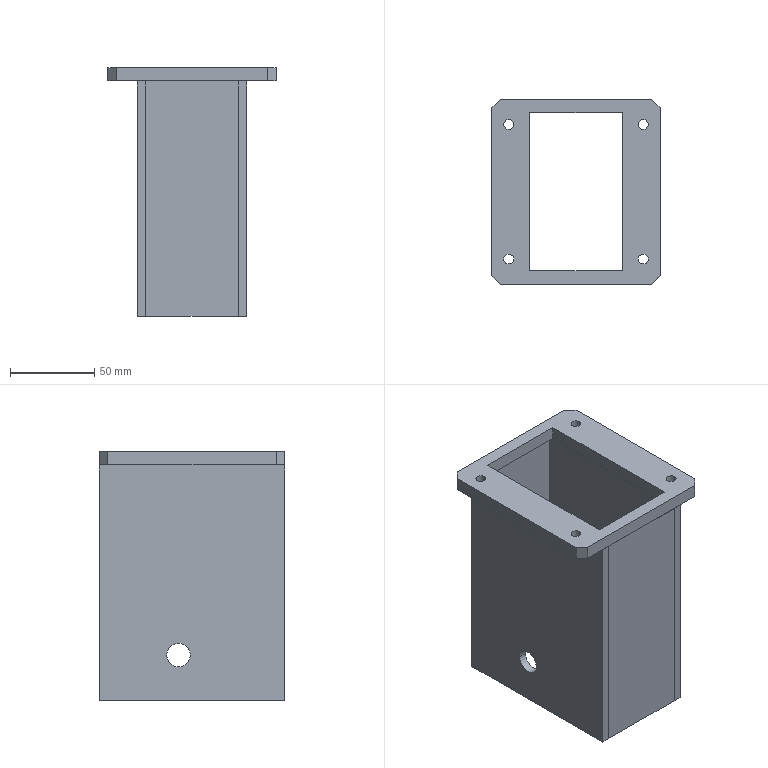Part | SolidWorks | features ICE 4, Chamfer 1, Extrusion 1, HoleWzd 1 | 5 solids | 50 faces | box 100 x 110 x 148 mm | volume 274855 mm3 | plane 38 | cylinder 12 | commonest cylinder face diameters 5.8 x8 14 x4
STEP:
#1=CARTESIAN_POINT('',(27.5,55.,0.));
#2=VERTEX_POINT('',#1);
#3=CARTESIAN_POINT('',(27.5,50.,0.));
#4=VERTEX_POINT('',#3);
#5=CARTESIAN_POINT('',(27.5,50.,0.));
#6=DIRECTION('',(0.,-1.,0.));
#7=VECTOR('',#6,1000.);
#8=LINE('',#5,#7);
#9=EDGE_CURVE('',#2,#4,#8,.T.);
#10=ORIENTED_EDGE('',*,*,#9,.T.);
#11=CARTESIAN_POINT('',(27.5,50.,-140.));
#12=VERTEX_POINT('',#11);
#13=CARTESIAN_POINT('',(27.5,50.,-140.));
#14=DIRECTION('',(0.,0.,1.));
#15=VECTOR('',#14,1000.);
#16=LINE('',#13,#15);
#17=EDGE_CURVE('',#12,#4,#16,.T.);
#18=ORIENTED_EDGE('',*,*,#17,.F.);
#19=CARTESIAN_POINT('',(27.5,55.,-140.));
#20=VERTEX_POINT('',#19);
#21=CARTESIAN_POINT('',(27.5,50.,-140.));
#22=DIRECTION('',(0.,-1.,0.));
#23=VECTOR('',#22,1000.);
#24=LINE('',#21,#23);
#25=EDGE_CURVE('',#20,#12,#24,.T.);
#26=ORIENTED_EDGE('',*,*,#25,.F.);
#27=CARTESIAN_POINT('',(27.5,55.,-140.));
#28=DIRECTION('',(0.,0.,1.));
#29=VECTOR('',#28,1000.);
#30=LINE('',#27,#29);
#31=EDGE_CURVE('',#20,#2,#30,.T.);
#32=ORIENTED_EDGE('',*,*,#31,.T.);
#33=EDGE_LOOP('',(#10,#18,#26,#32));
#34=FACE_OUTER_BOUND('',#33,.T.);
#35=CARTESIAN_POINT('',(27.5,50.,-140.));
#36=DIRECTION('',(-1.,0.,0.));
#37=DIRECTION('',(0.,-1.,0.));
#38=AXIS2_PLACEMENT_3D('',#35,#36,#37);
#39=PLANE('',#38);
#40=ADVANCED_FACE('',(#34),#39,.F.);
#41=CARTESIAN_POINT('',(-27.5,50.,0.));
#42=VERTEX_POINT('',#41);
#43=CARTESIAN_POINT('',(27.5,50.,0.));
#44=DIRECTION('',(-1.,0.,0.));
#45=VECTOR('',#44,1000.);
#46=LINE('',#43,#45);
#47=EDGE_CURVE('',#4,#42,#46,.T.);
#48=ORIENTED_EDGE('',*,*,#47,.T.);
#49=CARTESIAN_POINT('',(-27.5,50.,-140.));
#50=VERTEX_POINT('',#49);
#51=CARTESIAN_POINT('',(-27.5,50.,-140.));
#52=DIRECTION('',(0.,0.,1.));
#53=VECTOR('',#52,1000.);
#54=LINE('',#51,#53);
#55=EDGE_CURVE('',#50,#42,#54,.T.);
#56=ORIENTED_EDGE('',*,*,#55,.F.);
#57=CARTESIAN_POINT('',(27.5,50.,-140.));
#58=DIRECTION('',(-1.,0.,0.));
#59=VECTOR('',#58,1000.);
#60=LINE('',#57,#59);
#61=EDGE_CURVE('',#12,#50,#60,.T.);
#62=ORIENTED_EDGE('',*,*,#61,.F.);
#63=ORIENTED_EDGE('',*,*,#17,.T.);
#64=EDGE_LOOP('',(#48,#56,#62,#63));
#65=FACE_OUTER_BOUND('',#64,.T.);
#66=CARTESIAN_POINT('',(27.5,50.,-140.));
#67=DIRECTION('',(0.,1.,0.));
#68=DIRECTION('',(0.,0.,1.));
#69=AXIS2_PLACEMENT_3D('',#66,#67,#68);
#70=PLANE('',#69);
#71=ADVANCED_FACE('',(#65),#70,.F.);
#72=CARTESIAN_POINT('',(-27.5,55.,0.));
#73=VERTEX_POINT('',#72);
#74=CARTESIAN_POINT('',(-27.5,50.,0.));
#75=DIRECTION('',(0.,1.,0.));
#76=VECTOR('',#75,1000.);
#77=LINE('',#74,#76);
#78=EDGE_CURVE('',#42,#73,#77,.T.);
#79=ORIENTED_EDGE('',*,*,#78,.T.);
#80=CARTESIAN_POINT('',(-27.5,55.,-140.));
#81=VERTEX_POINT('',#80);
#82=CARTESIAN_POINT('',(-27.5,55.,-140.));
#83=DIRECTION('',(0.,0.,1.));
#84=VECTOR('',#83,1000.);
#85=LINE('',#82,#84);
#86=EDGE_CURVE('',#81,#73,#85,.T.);
#87=ORIENTED_EDGE('',*,*,#86,.F.);
#88=CARTESIAN_POINT('',(-27.5,50.,-140.));
#89=DIRECTION('',(0.,1.,0.));
#90=VECTOR('',#89,1000.);
#91=LINE('',#88,#90);
#92=EDGE_CURVE('',#50,#81,#91,.T.);
#93=ORIENTED_EDGE('',*,*,#92,.F.);
#94=ORIENTED_EDGE('',*,*,#55,.T.);
#95=EDGE_LOOP('',(#79,#87,#93,#94));
#96=FACE_OUTER_BOUND('',#95,.T.);
#97=CARTESIAN_POINT('',(-27.5,50.,-140.));
#98=DIRECTION('',(1.,0.,0.));
#99=DIRECTION('',(0.,0.,-1.));
#100=AXIS2_PLACEMENT_3D('',#97,#98,#99);
#101=PLANE('',#100);
#102=ADVANCED_FACE('',(#96),#101,.F.);
#103=CARTESIAN_POINT('',(27.5,55.,0.));
#104=DIRECTION('',(1.,0.,0.));
#105=VECTOR('',#104,1000.);
#106=LINE('',#103,#105);
#107=EDGE_CURVE('',#73,#2,#106,.T.);
#108=ORIENTED_EDGE('',*,*,#107,.T.);
#109=ORIENTED_EDGE('',*,*,#31,.F.);
#110=CARTESIAN_POINT('',(27.5,55.,-140.));
#111=DIRECTION('',(1.,0.,0.));
#112=VECTOR('',#111,1000.);
#113=LINE('',#110,#112);
#114=EDGE_CURVE('',#81,#20,#113,.T.);
#115=ORIENTED_EDGE('',*,*,#114,.F.);
#116=ORIENTED_EDGE('',*,*,#86,.T.);
#117=EDGE_LOOP('',(#108,#109,#115,#116));
#118=FACE_OUTER_BOUND('',#117,.T.);
#119=CARTESIAN_POINT('',(27.5,55.,-140.));
#120=DIRECTION('',(0.,-1.,0.));
#121=DIRECTION('',(0.,0.,-1.));
#122=AXIS2_PLACEMENT_3D('',#119,#120,#121);
#123=PLANE('',#122);
#124=ADVANCED_FACE('',(#118),#123,.F.);
#125=ORIENTED_EDGE('',*,*,#25,.T.);
#126=ORIENTED_EDGE('',*,*,#61,.T.);
#127=ORIENTED_EDGE('',*,*,#92,.T.);
#128=ORIENTED_EDGE('',*,*,#114,.T.);
#129=EDGE_LOOP('',(#125,#126,#127,#128));
#130=FACE_OUTER_BOUND('',#129,.T.);
#131=CARTESIAN_POINT('',(0.,0.,-140.));
#132=DIRECTION('',(0.,0.,1.));
#133=DIRECTION('',(1.,0.,0.));
#134=AXIS2_PLACEMENT_3D('',#131,#132,#133);
#135=PLANE('',#134);
#136=ADVANCED_FACE('',(#130),#135,.F.);
#137=ORIENTED_EDGE('',*,*,#9,.F.);
#138=ORIENTED_EDGE('',*,*,#107,.F.);
#139=ORIENTED_EDGE('',*,*,#78,.F.);
#140=ORIENTED_EDGE('',*,*,#47,.F.);
#141=EDGE_LOOP('',(#137,#138,#139,#140));
#142=FACE_OUTER_BOUND('',#141,.T.);
#143=CARTESIAN_POINT('',(0.,0.,0.));
#144=DIRECTION('',(0.,0.,1.));
#145=DIRECTION('',(1.,0.,0.));
#146=AXIS2_PLACEMENT_3D('',#143,#144,#145);
#147=PLANE('',#146);
#148=ADVANCED_FACE('',(#142),#147,.T.);
#149=CLOSED_SHELL('',(#40,#71,#102,#124,#136,#148));
#150=MANIFOLD_SOLID_BREP('',#149);
#151=CARTESIAN_POINT('',(-27.5,-50.,0.));
#152=VERTEX_POINT('',#151);
#153=CARTESIAN_POINT('',(27.5,-50.,0.));
#154=VERTEX_POINT('',#153);
#155=CARTESIAN_POINT('',(27.5,-50.,0.));
#156=DIRECTION('',(1.,0.,0.));
#157=VECTOR('',#156,1000.);
#158=LINE('',#155,#157);
#159=EDGE_CURVE('',#152,#154,#158,.T.);
#160=ORIENTED_EDGE('',*,*,#159,.T.);
#161=CARTESIAN_POINT('',(27.5,-50.,-140.));
#162=VERTEX_POINT('',#161);
#163=CARTESIAN_POINT('',(27.5,-50.,-140.));
#164=DIRECTION('',(0.,0.,1.));
#165=VECTOR('',#164,1000.);
#166=LINE('',#163,#165);
#167=EDGE_CURVE('',#162,#154,#166,.T.);
#168=ORIENTED_EDGE('',*,*,#167,.F.);
#169=CARTESIAN_POINT('',(-27.5,-50.,-140.));
#170=VERTEX_POINT('',#169);
#171=CARTESIAN_POINT('',(27.5,-50.,-140.));
#172=DIRECTION('',(1.,0.,0.));
#173=VECTOR('',#172,1000.);
#174=LINE('',#171,#173);
#175=EDGE_CURVE('',#170,#162,#174,.T.);
#176=ORIENTED_EDGE('',*,*,#175,.F.);
#177=CARTESIAN_POINT('',(-27.5,-50.,-140.));
#178=DIRECTION('',(0.,0.,1.));
#179=VECTOR('',#178,1000.);
#180=LINE('',#177,#179);
#181=EDGE_CURVE('',#170,#152,#180,.T.);
#182=ORIENTED_EDGE('',*,*,#181,.T.);
#183=EDGE_LOOP('',(#160,#168,#176,#182));
#184=FACE_OUTER_BOUND('',#183,.T.);
#185=CARTESIAN_POINT('',(27.5,-50.,-140.));
#186=DIRECTION('',(0.,-1.,0.));
#187=DIRECTION('',(0.,0.,-1.));
#188=AXIS2_PLACEMENT_3D('',#185,#186,#187);
#189=PLANE('',#188);
#190=ADVANCED_FACE('',(#184),#189,.F.);
#191=CARTESIAN_POINT('',(27.5,-55.,0.));
#192=VERTEX_POINT('',#191);
#193=CARTESIAN_POINT('',(27.5,-50.,0.));
#194=DIRECTION('',(0.,-1.,0.));
#195=VECTOR('',#194,1000.);
#196=LINE('',#193,#195);
#197=EDGE_CURVE('',#154,#192,#196,.T.);
#198=ORIENTED_EDGE('',*,*,#197,.T.);
#199=CARTESIAN_POINT('',(27.5,-55.,-140.));
#200=VERTEX_POINT('',#199);
#201=CARTESIAN_POINT('',(27.5,-55.,-140.));
#202=DIRECTION('',(0.,0.,1.));
#203=VECTOR('',#202,1000.);
#204=LINE('',#201,#203);
#205=EDGE_CURVE('',#200,#192,#204,.T.);
#206=ORIENTED_EDGE('',*,*,#205,.F.);
#207=CARTESIAN_POINT('',(27.5,-50.,-140.));
#208=DIRECTION('',(0.,-1.,0.));
#209=VECTOR('',#208,1000.);
#210=LINE('',#207,#209);
#211=EDGE_CURVE('',#162,#200,#210,.T.);
#212=ORIENTED_EDGE('',*,*,#211,.F.);
#213=ORIENTED_EDGE('',*,*,#167,.T.);
#214=EDGE_LOOP('',(#198,#206,#212,#213));
#215=FACE_OUTER_BOUND('',#214,.T.);
#216=CARTESIAN_POINT('',(27.5,-50.,-140.));
#217=DIRECTION('',(-1.,0.,0.));
#218=DIRECTION('',(0.,0.,1.));
#219=AXIS2_PLACEMENT_3D('',#216,#217,#218);
#220=PLANE('',#219);
#221=ADVANCED_FACE('',(#215),#220,.F.);
#222=CARTESIAN_POINT('',(-27.5,-55.,0.));
#223=VERTEX_POINT('',#222);
#224=CARTESIAN_POINT('',(27.5,-55.,0.));
#225=DIRECTION('',(-1.,0.,0.));
#226=VECTOR('',#225,1000.);
#227=LINE('',#224,#226);
#228=EDGE_CURVE('',#192,#223,#227,.T.);
#229=ORIENTED_EDGE('',*,*,#228,.T.);
#230=CARTESIAN_POINT('',(-27.5,-55.,-140.));
#231=VERTEX_POINT('',#230);
#232=CARTESIAN_POINT('',(-27.5,-55.,-140.));
#233=DIRECTION('',(0.,0.,1.));
#234=VECTOR('',#233,1000.);
#235=LINE('',#232,#234);
#236=EDGE_CURVE('',#231,#223,#235,.T.);
#237=ORIENTED_EDGE('',*,*,#236,.F.);
#238=CARTESIAN_POINT('',(27.5,-55.,-140.));
#239=DIRECTION('',(-1.,0.,0.));
#240=VECTOR('',#239,1000.);
#241=LINE('',#238,#240);
#242=EDGE_CURVE('',#200,#231,#241,.T.);
#243=ORIENTED_EDGE('',*,*,#242,.F.);
#244=ORIENTED_EDGE('',*,*,#205,.T.);
#245=EDGE_LOOP('',(#229,#237,#243,#244));
#246=FACE_OUTER_BOUND('',#245,.T.);
#247=CARTESIAN_POINT('',(27.5,-55.,-140.));
#248=DIRECTION('',(0.,1.,0.));
#249=DIRECTION('',(-1.,0.,0.));
#250=AXIS2_PLACEMENT_3D('',#247,#248,#249);
#251=PLANE('',#250);
#252=ADVANCED_FACE('',(#246),#251,.F.);
#253=CARTESIAN_POINT('',(-27.5,-50.,0.));
#254=DIRECTION('',(0.,1.,0.));
#255=VECTOR('',#254,1000.);
#256=LINE('',#253,#255);
#257=EDGE_CURVE('',#223,#152,#256,.T.);
#258=ORIENTED_EDGE('',*,*,#257,.T.);
#259=ORIENTED_EDGE('',*,*,#181,.F.);
#260=CARTESIAN_POINT('',(-27.5,-50.,-140.));
#261=DIRECTION('',(0.,1.,0.));
#262=VECTOR('',#261,1000.);
#263=LINE('',#260,#262);
#264=EDGE_CURVE('',#231,#170,#263,.T.);
#265=ORIENTED_EDGE('',*,*,#264,.F.);
#266=ORIENTED_EDGE('',*,*,#236,.T.);
#267=EDGE_LOOP('',(#258,#259,#265,#266));
#268=FACE_OUTER_BOUND('',#267,.T.);
#269=CARTESIAN_POINT('',(-27.5,-50.,-140.));
#270=DIRECTION('',(1.,0.,0.));
#271=DIRECTION('',(0.,0.,-1.));
#272=AXIS2_PLACEMENT_3D('',#269,#270,#271);
#273=PLANE('',#272);
#274=ADVANCED_FACE('',(#268),#273,.F.);
#275=ORIENTED_EDGE('',*,*,#175,.T.);
#276=ORIENTED_EDGE('',*,*,#211,.T.);
#277=ORIENTED_EDGE('',*,*,#242,.T.);
#278=ORIENTED_EDGE('',*,*,#264,.T.);
#279=EDGE_LOOP('',(#275,#276,#277,#278));
#280=FACE_OUTER_BOUND('',#279,.T.);
#281=CARTESIAN_POINT('',(0.,0.,-140.));
#282=DIRECTION('',(0.,0.,1.));
#283=DIRECTION('',(1.,0.,0.));
#284=AXIS2_PLACEMENT_3D('',#281,#282,#283);
#285=PLANE('',#284);
#286=ADVANCED_FACE('',(#280),#285,.F.);
#287=ORIENTED_EDGE('',*,*,#159,.F.);
#288=ORIENTED_EDGE('',*,*,#257,.F.);
#289=ORIENTED_EDGE('',*,*,#228,.F.);
#290=ORIENTED_EDGE('',*,*,#197,.F.);
#291=EDGE_LOOP('',(#287,#288,#289,#290));
#292=FACE_OUTER_BOUND('',#291,.T.);
#293=CARTESIAN_POINT('',(0.,0.,0.));
#294=DIRECTION('',(0.,0.,1.));
#295=DIRECTION('',(1.,0.,0.));
#296=AXIS2_PLACEMENT_3D('',#293,#294,#295);
#297=PLANE('',#296);
#298=ADVANCED_FACE('',(#292),#297,.T.);
#299=CLOSED_SHELL('',(#190,#221,#252,#274,#286,#298));
#300=MANIFOLD_SOLID_BREP('',#299);
#301=CARTESIAN_POINT('',(-42.9,40.,0.));
#302=VERTEX_POINT('',#301);
#303=CARTESIAN_POINT('',(-37.1,40.,0.));
#304=VERTEX_POINT('',#303);
#305=CARTESIAN_POINT('',(-40.,40.,0.));
#306=DIRECTION('',(0.,0.,1.));
#307=DIRECTION('',(1.,0.,0.));
#308=AXIS2_PLACEMENT_3D('',#305,#306,#307);
#309=CIRCLE('',#308,2.9);
#310=EDGE_CURVE('',#302,#304,#309,.T.);
#311=ORIENTED_EDGE('',*,*,#310,.F.);
#312=CARTESIAN_POINT('',(-42.9,40.,8.));
#313=VERTEX_POINT('',#312);
#314=CARTESIAN_POINT('',(-42.9,40.,8.));
#315=DIRECTION('',(0.,0.,1.));
#316=VECTOR('',#315,1000.);
#317=LINE('',#314,#316);
#318=EDGE_CURVE('',#302,#313,#317,.T.);
#319=ORIENTED_EDGE('',*,*,#318,.T.);
#320=CARTESIAN_POINT('',(-37.1,40.,8.));
#321=VERTEX_POINT('',#320);
#322=CARTESIAN_POINT('',(-40.,40.,8.));
#323=DIRECTION('',(0.,0.,1.));
#324=DIRECTION('',(1.,0.,0.));
#325=AXIS2_PLACEMENT_3D('',#322,#323,#324);
#326=CIRCLE('',#325,2.9);
#327=EDGE_CURVE('',#313,#321,#326,.T.);
#328=ORIENTED_EDGE('',*,*,#327,.T.);
#329=CARTESIAN_POINT('',(-37.1,40.,8.));
#330=DIRECTION('',(0.,0.,1.));
#331=VECTOR('',#330,1000.);
#332=LINE('',#329,#331);
#333=EDGE_CURVE('',#304,#321,#332,.T.);
#334=ORIENTED_EDGE('',*,*,#333,.F.);
#335=EDGE_LOOP('',(#311,#319,#328,#334));
#336=FACE_OUTER_BOUND('',#335,.T.);
#337=CARTESIAN_POINT('',(-40.,40.,8.));
#338=DIRECTION('',(0.,0.,1.));
#339=DIRECTION('',(1.,0.,0.));
#340=AXIS2_PLACEMENT_3D('',#337,#338,#339);
#341=CYLINDRICAL_SURFACE('',#340,2.9);
#342=ADVANCED_FACE('',(#336),#341,.F.);
#343=CARTESIAN_POINT('',(-42.9,-40.,0.));
#344=VERTEX_POINT('',#343);
#345=CARTESIAN_POINT('',(-37.1,-40.,0.));
#346=VERTEX_POINT('',#345);
#347=CARTESIAN_POINT('',(-40.,-40.,0.));
#348=DIRECTION('',(0.,0.,1.));
#349=DIRECTION('',(1.,0.,0.));
#350=AXIS2_PLACEMENT_3D('',#347,#348,#349);
#351=CIRCLE('',#350,2.9);
#352=EDGE_CURVE('',#344,#346,#351,.T.);
#353=ORIENTED_EDGE('',*,*,#352,.F.);
#354=CARTESIAN_POINT('',(-42.9,-40.,8.));
#355=VERTEX_POINT('',#354);
#356=CARTESIAN_POINT('',(-42.9,-40.,8.));
#357=DIRECTION('',(0.,0.,1.));
#358=VECTOR('',#357,1000.);
#359=LINE('',#356,#358);
#360=EDGE_CURVE('',#344,#355,#359,.T.);
#361=ORIENTED_EDGE('',*,*,#360,.T.);
#362=CARTESIAN_POINT('',(-37.1,-40.,8.));
#363=VERTEX_POINT('',#362);
#364=CARTESIAN_POINT('',(-40.,-40.,8.));
#365=DIRECTION('',(0.,0.,1.));
#366=DIRECTION('',(1.,0.,0.));
#367=AXIS2_PLACEMENT_3D('',#364,#365,#366);
#368=CIRCLE('',#367,2.9);
#369=EDGE_CURVE('',#355,#363,#368,.T.);
#370=ORIENTED_EDGE('',*,*,#369,.T.);
#371=CARTESIAN_POINT('',(-37.1,-40.,8.));
#372=DIRECTION('',(0.,0.,1.));
#373=VECTOR('',#372,1000.);
#374=LINE('',#371,#373);
#375=EDGE_CURVE('',#346,#363,#374,.T.);
#376=ORIENTED_EDGE('',*,*,#375,.F.);
#377=EDGE_LOOP('',(#353,#361,#370,#376));
#378=FACE_OUTER_BOUND('',#377,.T.);
#379=CARTESIAN_POINT('',(-40.,-40.,8.));
#380=DIRECTION('',(0.,0.,1.));
#381=DIRECTION('',(1.,0.,0.));
#382=AXIS2_PLACEMENT_3D('',#379,#380,#381);
#383=CYLINDRICAL_SURFACE('',#382,2.9);
#384=ADVANCED_FACE('',(#378),#383,.F.);
#385=CARTESIAN_POINT('',(37.1,-40.,0.));
#386=VERTEX_POINT('',#385);
#387=CARTESIAN_POINT('',(42.9,-40.,0.));
#388=VERTEX_POINT('',#387);
#389=CARTESIAN_POINT('',(40.,-40.,0.));
#390=DIRECTION('',(0.,0.,1.));
#391=DIRECTION('',(1.,0.,0.));
#392=AXIS2_PLACEMENT_3D('',#389,#390,#391);
#393=CIRCLE('',#392,2.9);
#394=EDGE_CURVE('',#386,#388,#393,.T.);
#395=ORIENTED_EDGE('',*,*,#394,.F.);
#396=CARTESIAN_POINT('',(37.1,-40.,8.));
#397=VERTEX_POINT('',#396);
#398=CARTESIAN_POINT('',(37.1,-40.,8.));
#399=DIRECTION('',(0.,0.,1.));
#400=VECTOR('',#399,1000.);
#401=LINE('',#398,#400);
#402=EDGE_CURVE('',#386,#397,#401,.T.);
#403=ORIENTED_EDGE('',*,*,#402,.T.);
#404=CARTESIAN_POINT('',(42.9,-40.,8.));
#405=VERTEX_POINT('',#404);
#406=CARTESIAN_POINT('',(40.,-40.,8.));
#407=DIRECTION('',(0.,0.,1.));
#408=DIRECTION('',(1.,0.,0.));
#409=AXIS2_PLACEMENT_3D('',#406,#407,#408);
#410=CIRCLE('',#409,2.9);
#411=EDGE_CURVE('',#397,#405,#410,.T.);
#412=ORIENTED_EDGE('',*,*,#411,.T.);
#413=CARTESIAN_POINT('',(42.9,-40.,8.));
#414=DIRECTION('',(0.,0.,1.));
#415=VECTOR('',#414,1000.);
#416=LINE('',#413,#415);
#417=EDGE_CURVE('',#388,#405,#416,.T.);
#418=ORIENTED_EDGE('',*,*,#417,.F.);
#419=EDGE_LOOP('',(#395,#403,#412,#418));
#420=FACE_OUTER_BOUND('',#419,.T.);
#421=CARTESIAN_POINT('',(40.,-40.,8.));
#422=DIRECTION('',(0.,0.,1.));
#423=DIRECTION('',(1.,0.,0.));
#424=AXIS2_PLACEMENT_3D('',#421,#422,#423);
#425=CYLINDRICAL_SURFACE('',#424,2.9);
#426=ADVANCED_FACE('',(#420),#425,.F.);
#427=CARTESIAN_POINT('',(37.1,40.,0.));
#428=VERTEX_POINT('',#427);
#429=CARTESIAN_POINT('',(42.9,40.,0.));
#430=VERTEX_POINT('',#429);
#431=CARTESIAN_POINT('',(40.,40.,0.));
#432=DIRECTION('',(0.,0.,1.));
#433=DIRECTION('',(1.,0.,0.));
#434=AXIS2_PLACEMENT_3D('',#431,#432,#433);
#435=CIRCLE('',#434,2.9);
#436=EDGE_CURVE('',#428,#430,#435,.T.);
#437=ORIENTED_EDGE('',*,*,#436,.F.);
#438=CARTESIAN_POINT('',(37.1,40.,8.));
#439=VERTEX_POINT('',#438);
#440=CARTESIAN_POINT('',(37.1,40.,8.));
#441=DIRECTION('',(0.,0.,1.));
#442=VECTOR('',#441,1000.);
#443=LINE('',#440,#442);
#444=EDGE_CURVE('',#428,#439,#443,.T.);
#445=ORIENTED_EDGE('',*,*,#444,.T.);
#446=CARTESIAN_POINT('',(42.9,40.,8.));
#447=VERTEX_POINT('',#446);
#448=CARTESIAN_POINT('',(40.,40.,8.));
#449=DIRECTION('',(0.,0.,1.));
#450=DIRECTION('',(1.,0.,0.));
#451=AXIS2_PLACEMENT_3D('',#448,#449,#450);
#452=CIRCLE('',#451,2.9);
#453=EDGE_CURVE('',#439,#447,#452,.T.);
#454=ORIENTED_EDGE('',*,*,#453,.T.);
#455=CARTESIAN_POINT('',(42.9,40.,8.));
#456=DIRECTION('',(0.,0.,1.));
#457=VECTOR('',#456,1000.);
#458=LINE('',#455,#457);
#459=EDGE_CURVE('',#430,#447,#458,.T.);
#460=ORIENTED_EDGE('',*,*,#459,.F.);
#461=EDGE_LOOP('',(#437,#445,#454,#460));
#462=FACE_OUTER_BOUND('',#461,.T.);
#463=CARTESIAN_POINT('',(40.,40.,8.));
#464=DIRECTION('',(0.,0.,1.));
#465=DIRECTION('',(1.,0.,0.));
#466=AXIS2_PLACEMENT_3D('',#463,#464,#465);
#467=CYLINDRICAL_SURFACE('',#466,2.9);
#468=ADVANCED_FACE('',(#462),#467,.F.);
#469=CARTESIAN_POINT('',(50.,-50.,8.));
#470=VERTEX_POINT('',#469);
#471=CARTESIAN_POINT('',(50.,50.,8.));
#472=VERTEX_POINT('',#471);
#473=CARTESIAN_POINT('',(50.,55.,8.));
#474=DIRECTION('',(0.,1.,0.));
#475=VECTOR('',#474,1000.);
#476=LINE('',#473,#475);
#477=EDGE_CURVE('',#470,#472,#476,.T.);
#478=ORIENTED_EDGE('',*,*,#477,.F.);
#479=CARTESIAN_POINT('',(50.,-50.,0.));
#480=VERTEX_POINT('',#479);
#481=CARTESIAN_POINT('',(50.,-50.,8.));
#482=DIRECTION('',(0.,0.,-1.));
#483=VECTOR('',#482,1000.);
#484=LINE('',#481,#483);
#485=EDGE_CURVE('',#470,#480,#484,.T.);
#486=ORIENTED_EDGE('',*,*,#485,.T.);
#487=CARTESIAN_POINT('',(50.,50.,0.));
#488=VERTEX_POINT('',#487);
#489=CARTESIAN_POINT('',(50.,55.,0.));
#490=DIRECTION('',(0.,1.,0.));
#491=VECTOR('',#490,1000.);
#492=LINE('',#489,#491);
#493=EDGE_CURVE('',#480,#488,#492,.T.);
#494=ORIENTED_EDGE('',*,*,#493,.T.);
#495=CARTESIAN_POINT('',(50.,50.,8.));
#496=DIRECTION('',(0.,0.,1.));
#497=VECTOR('',#496,1000.);
#498=LINE('',#495,#497);
#499=EDGE_CURVE('',#488,#472,#498,.T.);
#500=ORIENTED_EDGE('',*,*,#499,.T.);
#501=EDGE_LOOP('',(#478,#486,#494,#500));
#502=FACE_OUTER_BOUND('',#501,.T.);
#503=CARTESIAN_POINT('',(50.,55.,8.));
#504=DIRECTION('',(-1.,0.,0.));
#505=DIRECTION('',(0.,-1.,0.));
#506=AXIS2_PLACEMENT_3D('',#503,#504,#505);
#507=PLANE('',#506);
#508=ADVANCED_FACE('',(#502),#507,.F.);
#509=CARTESIAN_POINT('',(45.,55.,0.));
#510=VERTEX_POINT('',#509);
#511=CARTESIAN_POINT('',(-45.,55.,0.));
#512=VERTEX_POINT('',#511);
#513=CARTESIAN_POINT('',(-50.,55.,0.));
#514=DIRECTION('',(-1.,0.,0.));
#515=VECTOR('',#514,1000.);
#516=LINE('',#513,#515);
#517=EDGE_CURVE('',#510,#512,#516,.T.);
#518=ORIENTED_EDGE('',*,*,#517,.T.);
#519=CARTESIAN_POINT('',(-45.,55.,8.));
#520=VERTEX_POINT('',#519);
#521=CARTESIAN_POINT('',(-45.,55.,8.));
#522=DIRECTION('',(0.,0.,1.));
#523=VECTOR('',#522,1000.);
#524=LINE('',#521,#523);
#525=EDGE_CURVE('',#512,#520,#524,.T.);
#526=ORIENTED_EDGE('',*,*,#525,.T.);
#527=CARTESIAN_POINT('',(45.,55.,8.));
#528=VERTEX_POINT('',#527);
#529=CARTESIAN_POINT('',(-50.,55.,8.));
#530=DIRECTION('',(-1.,0.,0.));
#531=VECTOR('',#530,1000.);
#532=LINE('',#529,#531);
#533=EDGE_CURVE('',#528,#520,#532,.T.);
#534=ORIENTED_EDGE('',*,*,#533,.F.);
#535=CARTESIAN_POINT('',(45.,55.,8.));
#536=DIRECTION('',(0.,0.,-1.));
#537=VECTOR('',#536,1000.);
#538=LINE('',#535,#537);
#539=EDGE_CURVE('',#528,#510,#538,.T.);
#540=ORIENTED_EDGE('',*,*,#539,.T.);
#541=EDGE_LOOP('',(#518,#526,#534,#540));
#542=FACE_OUTER_BOUND('',#541,.T.);
#543=CARTESIAN_POINT('',(-50.,55.,8.));
#544=DIRECTION('',(0.,-1.,0.));
#545=DIRECTION('',(0.,0.,-1.));
#546=AXIS2_PLACEMENT_3D('',#543,#544,#545);
#547=PLANE('',#546);
#548=ADVANCED_FACE('',(#542),#547,.F.);
#549=CARTESIAN_POINT('',(-50.,50.,0.));
#550=VERTEX_POINT('',#549);
#551=CARTESIAN_POINT('',(-50.,-50.,0.));
#552=VERTEX_POINT('',#551);
#553=CARTESIAN_POINT('',(-50.,55.,0.));
#554=DIRECTION('',(0.,-1.,0.));
#555=VECTOR('',#554,1000.);
#556=LINE('',#553,#555);
#557=EDGE_CURVE('',#550,#552,#556,.T.);
#558=ORIENTED_EDGE('',*,*,#557,.T.);
#559=CARTESIAN_POINT('',(-50.,-50.,8.));
#560=VERTEX_POINT('',#559);
#561=CARTESIAN_POINT('',(-50.,-50.,8.));
#562=DIRECTION('',(0.,0.,1.));
#563=VECTOR('',#562,1000.);
#564=LINE('',#561,#563);
#565=EDGE_CURVE('',#552,#560,#564,.T.);
#566=ORIENTED_EDGE('',*,*,#565,.T.);
#567=CARTESIAN_POINT('',(-50.,50.,8.));
#568=VERTEX_POINT('',#567);
#569=CARTESIAN_POINT('',(-50.,55.,8.));
#570=DIRECTION('',(0.,-1.,0.));
#571=VECTOR('',#570,1000.);
#572=LINE('',#569,#571);
#573=EDGE_CURVE('',#568,#560,#572,.T.);
#574=ORIENTED_EDGE('',*,*,#573,.F.);
#575=CARTESIAN_POINT('',(-50.,50.,8.));
#576=DIRECTION('',(0.,0.,-1.));
#577=VECTOR('',#576,1000.);
#578=LINE('',#575,#577);
#579=EDGE_CURVE('',#568,#550,#578,.T.);
#580=ORIENTED_EDGE('',*,*,#579,.T.);
#581=EDGE_LOOP('',(#558,#566,#574,#580));
#582=FACE_OUTER_BOUND('',#581,.T.);
#583=CARTESIAN_POINT('',(-50.,55.,8.));
#584=DIRECTION('',(1.,0.,0.));
#585=DIRECTION('',(0.,1.,0.));
#586=AXIS2_PLACEMENT_3D('',#583,#584,#585);
#587=PLANE('',#586);
#588=ADVANCED_FACE('',(#582),#587,.F.);
#589=CARTESIAN_POINT('',(-45.,-55.,0.));
#590=VERTEX_POINT('',#589);
#591=CARTESIAN_POINT('',(45.,-55.,0.));
#592=VERTEX_POINT('',#591);
#593=CARTESIAN_POINT('',(-50.,-55.,0.));
#594=DIRECTION('',(1.,0.,0.));
#595=VECTOR('',#594,1000.);
#596=LINE('',#593,#595);
#597=EDGE_CURVE('',#590,#592,#596,.T.);
#598=ORIENTED_EDGE('',*,*,#597,.T.);
#599=CARTESIAN_POINT('',(45.,-55.,8.));
#600=VERTEX_POINT('',#599);
#601=CARTESIAN_POINT('',(45.,-55.,8.));
#602=DIRECTION('',(0.,0.,1.));
#603=VECTOR('',#602,1000.);
#604=LINE('',#601,#603);
#605=EDGE_CURVE('',#592,#600,#604,.T.);
#606=ORIENTED_EDGE('',*,*,#605,.T.);
#607=CARTESIAN_POINT('',(-45.,-55.,8.));
#608=VERTEX_POINT('',#607);
#609=CARTESIAN_POINT('',(-50.,-55.,8.));
#610=DIRECTION('',(1.,0.,0.));
#611=VECTOR('',#610,1000.);
#612=LINE('',#609,#611);
#613=EDGE_CURVE('',#608,#600,#612,.T.);
#614=ORIENTED_EDGE('',*,*,#613,.F.);
#615=CARTESIAN_POINT('',(-45.,-55.,8.));
#616=DIRECTION('',(0.,0.,-1.));
#617=VECTOR('',#616,1000.);
#618=LINE('',#615,#617);
#619=EDGE_CURVE('',#608,#590,#618,.T.);
#620=ORIENTED_EDGE('',*,*,#619,.T.);
#621=EDGE_LOOP('',(#598,#606,#614,#620));
#622=FACE_OUTER_BOUND('',#621,.T.);
#623=CARTESIAN_POINT('',(-50.,-55.,8.));
#624=DIRECTION('',(0.,1.,0.));
#625=DIRECTION('',(0.,0.,1.));
#626=AXIS2_PLACEMENT_3D('',#623,#624,#625);
#627=PLANE('',#626);
#628=ADVANCED_FACE('',(#622),#627,.F.);
#629=CARTESIAN_POINT('',(-40.,40.,8.));
#630=DIRECTION('',(0.,0.,1.));
#631=DIRECTION('',(1.,0.,0.));
#632=AXIS2_PLACEMENT_3D('',#629,#630,#631);
#633=CIRCLE('',#632,2.9);
#634=EDGE_CURVE('',#321,#313,#633,.T.);
#635=ORIENTED_EDGE('',*,*,#634,.F.);
#636=ORIENTED_EDGE('',*,*,#327,.F.);
#637=EDGE_LOOP('',(#635,#636));
#638=FACE_BOUND('',#637,.T.);
#639=CARTESIAN_POINT('',(-40.,-40.,8.));
#640=DIRECTION('',(0.,0.,1.));
#641=DIRECTION('',(1.,0.,0.));
#642=AXIS2_PLACEMENT_3D('',#639,#640,#641);
#643=CIRCLE('',#642,2.9);
#644=EDGE_CURVE('',#363,#355,#643,.T.);
#645=ORIENTED_EDGE('',*,*,#644,.F.);
#646=ORIENTED_EDGE('',*,*,#369,.F.);
#647=EDGE_LOOP('',(#645,#646));
#648=FACE_BOUND('',#647,.T.);
#649=CARTESIAN_POINT('',(40.,-40.,8.));
#650=DIRECTION('',(0.,0.,1.));
#651=DIRECTION('',(1.,0.,0.));
#652=AXIS2_PLACEMENT_3D('',#649,#650,#651);
#653=CIRCLE('',#652,2.9);
#654=EDGE_CURVE('',#405,#397,#653,.T.);
#655=ORIENTED_EDGE('',*,*,#654,.F.);
#656=ORIENTED_EDGE('',*,*,#411,.F.);
#657=EDGE_LOOP('',(#655,#656));
#658=FACE_BOUND('',#657,.T.);
#659=CARTESIAN_POINT('',(40.,40.,8.));
#660=DIRECTION('',(0.,0.,1.));
#661=DIRECTION('',(1.,0.,0.));
#662=AXIS2_PLACEMENT_3D('',#659,#660,#661);
#663=CIRCLE('',#662,2.9);
#664=EDGE_CURVE('',#447,#439,#663,.T.);
#665=ORIENTED_EDGE('',*,*,#664,.F.);
#666=ORIENTED_EDGE('',*,*,#453,.F.);
#667=EDGE_LOOP('',(#665,#666));
#668=FACE_BOUND('',#667,.T.);
#669=CARTESIAN_POINT('',(27.5,-47.,8.));
#670=VERTEX_POINT('',#669);
#671=CARTESIAN_POINT('',(27.5,47.,8.));
#672=VERTEX_POINT('',#671);
#673=CARTESIAN_POINT('',(27.5,47.,8.));
#674=DIRECTION('',(0.,1.,0.));
#675=VECTOR('',#674,1000.);
#676=LINE('',#673,#675);
#677=EDGE_CURVE('',#670,#672,#676,.T.);
#678=ORIENTED_EDGE('',*,*,#677,.F.);
#679=CARTESIAN_POINT('',(-27.5,-47.,8.));
#680=VERTEX_POINT('',#679);
#681=CARTESIAN_POINT('',(-27.5,-47.,8.));
#682=DIRECTION('',(1.,0.,0.));
#683=VECTOR('',#682,1000.);
#684=LINE('',#681,#683);
#685=EDGE_CURVE('',#680,#670,#684,.T.);
#686=ORIENTED_EDGE('',*,*,#685,.F.);
#687=CARTESIAN_POINT('',(-27.5,47.,8.));
#688=VERTEX_POINT('',#687);
#689=CARTESIAN_POINT('',(-27.5,47.,8.));
#690=DIRECTION('',(0.,-1.,0.));
#691=VECTOR('',#690,1000.);
#692=LINE('',#689,#691);
#693=EDGE_CURVE('',#688,#680,#692,.T.);
#694=ORIENTED_EDGE('',*,*,#693,.F.);
#695=CARTESIAN_POINT('',(-27.5,47.,8.));
#696=DIRECTION('',(-1.,0.,0.));
#697=VECTOR('',#696,1000.);
#698=LINE('',#695,#697);
#699=EDGE_CURVE('',#672,#688,#698,.T.);
#700=ORIENTED_EDGE('',*,*,#699,.F.);
#701=EDGE_LOOP('',(#678,#686,#694,#700));
#702=FACE_BOUND('',#701,.T.);
#703=ORIENTED_EDGE('',*,*,#613,.T.);
#704=CARTESIAN_POINT('',(50.,-50.,8.));
#705=DIRECTION('',(0.7071,0.7071,0.));
#706=VECTOR('',#705,1000.);
#707=LINE('',#704,#706);
#708=EDGE_CURVE('',#600,#470,#707,.T.);
#709=ORIENTED_EDGE('',*,*,#708,.T.);
#710=ORIENTED_EDGE('',*,*,#477,.T.);
#711=CARTESIAN_POINT('',(50.,50.,8.));
#712=DIRECTION('',(-0.7071,0.7071,0.));
#713=VECTOR('',#712,1000.);
#714=LINE('',#711,#713);
#715=EDGE_CURVE('',#472,#528,#714,.T.);
#716=ORIENTED_EDGE('',*,*,#715,.T.);
#717=ORIENTED_EDGE('',*,*,#533,.T.);
#718=CARTESIAN_POINT('',(-50.,50.,8.));
#719=DIRECTION('',(-0.7071,-0.7071,0.));
#720=VECTOR('',#719,1000.);
#721=LINE('',#718,#720);
#722=EDGE_CURVE('',#520,#568,#721,.T.);
#723=ORIENTED_EDGE('',*,*,#722,.T.);
#724=ORIENTED_EDGE('',*,*,#573,.T.);
#725=CARTESIAN_POINT('',(-50.,-50.,8.));
#726=DIRECTION('',(0.7071,-0.7071,0.));
#727=VECTOR('',#726,1000.);
#728=LINE('',#725,#727);
#729=EDGE_CURVE('',#560,#608,#728,.T.);
#730=ORIENTED_EDGE('',*,*,#729,.T.);
#731=EDGE_LOOP('',(#703,#709,#710,#716,#717,#723,#724,#730));
#732=FACE_OUTER_BOUND('',#731,.T.);
#733=CARTESIAN_POINT('',(0.,0.,8.));
#734=DIRECTION('',(0.,0.,1.));
#735=DIRECTION('',(1.,0.,0.));
#736=AXIS2_PLACEMENT_3D('',#733,#734,#735);
#737=PLANE('',#736);
#738=ADVANCED_FACE('',(#638,#648,#658,#668,#702,#732),#737,.T.);
#739=CARTESIAN_POINT('',(-40.,40.,0.));
#740=DIRECTION('',(0.,0.,1.));
#741=DIRECTION('',(1.,0.,0.));
#742=AXIS2_PLACEMENT_3D('',#739,#740,#741);
#743=CIRCLE('',#742,2.9);
#744=EDGE_CURVE('',#304,#302,#743,.T.);
#745=ORIENTED_EDGE('',*,*,#744,.T.);
#746=ORIENTED_EDGE('',*,*,#310,.T.);
#747=EDGE_LOOP('',(#745,#746));
#748=FACE_BOUND('',#747,.T.);
#749=CARTESIAN_POINT('',(-40.,-40.,0.));
#750=DIRECTION('',(0.,0.,1.));
#751=DIRECTION('',(1.,0.,0.));
#752=AXIS2_PLACEMENT_3D('',#749,#750,#751);
#753=CIRCLE('',#752,2.9);
#754=EDGE_CURVE('',#346,#344,#753,.T.);
#755=ORIENTED_EDGE('',*,*,#754,.T.);
#756=ORIENTED_EDGE('',*,*,#352,.T.);
#757=EDGE_LOOP('',(#755,#756));
#758=FACE_BOUND('',#757,.T.);
#759=CARTESIAN_POINT('',(40.,-40.,0.));
#760=DIRECTION('',(0.,0.,1.));
#761=DIRECTION('',(1.,0.,0.));
#762=AXIS2_PLACEMENT_3D('',#759,#760,#761);
#763=CIRCLE('',#762,2.9);
#764=EDGE_CURVE('',#388,#386,#763,.T.);
#765=ORIENTED_EDGE('',*,*,#764,.T.);
#766=ORIENTED_EDGE('',*,*,#394,.T.);
#767=EDGE_LOOP('',(#765,#766));
#768=FACE_BOUND('',#767,.T.);
#769=CARTESIAN_POINT('',(40.,40.,0.));
#770=DIRECTION('',(0.,0.,1.));
#771=DIRECTION('',(1.,0.,0.));
#772=AXIS2_PLACEMENT_3D('',#769,#770,#771);
#773=CIRCLE('',#772,2.9);
#774=EDGE_CURVE('',#430,#428,#773,.T.);
#775=ORIENTED_EDGE('',*,*,#774,.T.);
#776=ORIENTED_EDGE('',*,*,#436,.T.);
#777=EDGE_LOOP('',(#775,#776));
#778=FACE_BOUND('',#777,.T.);
#779=CARTESIAN_POINT('',(-27.5,-47.,0.));
#780=VERTEX_POINT('',#779);
#781=CARTESIAN_POINT('',(27.5,-47.,0.));
#782=VERTEX_POINT('',#781);
#783=CARTESIAN_POINT('',(-27.5,-47.,0.));
#784=DIRECTION('',(1.,0.,0.));
#785=VECTOR('',#784,1000.);
#786=LINE('',#783,#785);
#787=EDGE_CURVE('',#780,#782,#786,.T.);
#788=ORIENTED_EDGE('',*,*,#787,.T.);
#789=CARTESIAN_POINT('',(27.5,47.,0.));
#790=VERTEX_POINT('',#789);
#791=CARTESIAN_POINT('',(27.5,47.,0.));
#792=DIRECTION('',(0.,1.,0.));
#793=VECTOR('',#792,1000.);
#794=LINE('',#791,#793);
#795=EDGE_CURVE('',#782,#790,#794,.T.);
#796=ORIENTED_EDGE('',*,*,#795,.T.);
#797=CARTESIAN_POINT('',(-27.5,47.,0.));
#798=VERTEX_POINT('',#797);
#799=CARTESIAN_POINT('',(-27.5,47.,0.));
#800=DIRECTION('',(-1.,0.,0.));
#801=VECTOR('',#800,1000.);
#802=LINE('',#799,#801);
#803=EDGE_CURVE('',#790,#798,#802,.T.);
#804=ORIENTED_EDGE('',*,*,#803,.T.);
#805=CARTESIAN_POINT('',(-27.5,47.,0.));
#806=DIRECTION('',(0.,-1.,0.));
#807=VECTOR('',#806,1000.);
#808=LINE('',#805,#807);
#809=EDGE_CURVE('',#798,#780,#808,.T.);
#810=ORIENTED_EDGE('',*,*,#809,.T.);
#811=EDGE_LOOP('',(#788,#796,#804,#810));
#812=FACE_BOUND('',#811,.T.);
#813=ORIENTED_EDGE('',*,*,#493,.F.);
#814=CARTESIAN_POINT('',(50.,-50.,0.));
#815=DIRECTION('',(-0.7071,-0.7071,0.));
#816=VECTOR('',#815,1000.);
#817=LINE('',#814,#816);
#818=EDGE_CURVE('',#480,#592,#817,.T.);
#819=ORIENTED_EDGE('',*,*,#818,.T.);
#820=ORIENTED_EDGE('',*,*,#597,.F.);
#821=CARTESIAN_POINT('',(-45.,-55.,0.));
#822=DIRECTION('',(-0.7071,0.7071,0.));
#823=VECTOR('',#822,1000.);
#824=LINE('',#821,#823);
#825=EDGE_CURVE('',#590,#552,#824,.T.);
#826=ORIENTED_EDGE('',*,*,#825,.T.);
#827=ORIENTED_EDGE('',*,*,#557,.F.);
#828=CARTESIAN_POINT('',(-50.,50.,0.));
#829=DIRECTION('',(0.7071,0.7071,0.));
#830=VECTOR('',#829,1000.);
#831=LINE('',#828,#830);
#832=EDGE_CURVE('',#550,#512,#831,.T.);
#833=ORIENTED_EDGE('',*,*,#832,.T.);
#834=ORIENTED_EDGE('',*,*,#517,.F.);
#835=CARTESIAN_POINT('',(45.,55.,0.));
#836=DIRECTION('',(0.7071,-0.7071,0.));
#837=VECTOR('',#836,1000.);
#838=LINE('',#835,#837);
#839=EDGE_CURVE('',#510,#488,#838,.T.);
#840=ORIENTED_EDGE('',*,*,#839,.T.);
#841=EDGE_LOOP('',(#813,#819,#820,#826,#827,#833,#834,#840));
#842=FACE_OUTER_BOUND('',#841,.T.);
#843=CARTESIAN_POINT('',(0.,0.,0.));
#844=DIRECTION('',(0.,0.,1.));
#845=DIRECTION('',(1.,0.,0.));
#846=AXIS2_PLACEMENT_3D('',#843,#844,#845);
#847=PLANE('',#846);
#848=ADVANCED_FACE('',(#748,#758,#768,#778,#812,#842),#847,.F.);
#849=ORIENTED_EDGE('',*,*,#677,.T.);
#850=CARTESIAN_POINT('',(27.5,47.,0.));
#851=DIRECTION('',(0.,0.,1.));
#852=VECTOR('',#851,1000.);
#853=LINE('',#850,#852);
#854=EDGE_CURVE('',#790,#672,#853,.T.);
#855=ORIENTED_EDGE('',*,*,#854,.F.);
#856=ORIENTED_EDGE('',*,*,#795,.F.);
#857=CARTESIAN_POINT('',(27.5,-47.,0.));
#858=DIRECTION('',(0.,0.,1.));
#859=VECTOR('',#858,1000.);
#860=LINE('',#857,#859);
#861=EDGE_CURVE('',#782,#670,#860,.T.);
#862=ORIENTED_EDGE('',*,*,#861,.T.);
#863=EDGE_LOOP('',(#849,#855,#856,#862));
#864=FACE_OUTER_BOUND('',#863,.T.);
#865=CARTESIAN_POINT('',(27.5,47.,0.));
#866=DIRECTION('',(1.,0.,0.));
#867=DIRECTION('',(0.,0.,-1.));
#868=AXIS2_PLACEMENT_3D('',#865,#866,#867);
#869=PLANE('',#868);
#870=ADVANCED_FACE('',(#864),#869,.F.);
#871=ORIENTED_EDGE('',*,*,#685,.T.);
#872=ORIENTED_EDGE('',*,*,#861,.F.);
#873=ORIENTED_EDGE('',*,*,#787,.F.);
#874=CARTESIAN_POINT('',(-27.5,-47.,0.));
#875=DIRECTION('',(0.,0.,1.));
#876=VECTOR('',#875,1000.);
#877=LINE('',#874,#876);
#878=EDGE_CURVE('',#780,#680,#877,.T.);
#879=ORIENTED_EDGE('',*,*,#878,.T.);
#880=EDGE_LOOP('',(#871,#872,#873,#879));
#881=FACE_OUTER_BOUND('',#880,.T.);
#882=CARTESIAN_POINT('',(-27.5,-47.,0.));
#883=DIRECTION('',(0.,-1.,0.));
#884=DIRECTION('',(0.,0.,-1.));
#885=AXIS2_PLACEMENT_3D('',#882,#883,#884);
#886=PLANE('',#885);
#887=ADVANCED_FACE('',(#881),#886,.F.);
#888=ORIENTED_EDGE('',*,*,#693,.T.);
#889=ORIENTED_EDGE('',*,*,#878,.F.);
#890=ORIENTED_EDGE('',*,*,#809,.F.);
#891=CARTESIAN_POINT('',(-27.5,47.,0.));
#892=DIRECTION('',(0.,0.,1.));
#893=VECTOR('',#892,1000.);
#894=LINE('',#891,#893);
#895=EDGE_CURVE('',#798,#688,#894,.T.);
#896=ORIENTED_EDGE('',*,*,#895,.T.);
#897=EDGE_LOOP('',(#888,#889,#890,#896));
#898=FACE_OUTER_BOUND('',#897,.T.);
#899=CARTESIAN_POINT('',(-27.5,47.,0.));
#900=DIRECTION('',(-1.,0.,0.));
#901=DIRECTION('',(0.,0.,1.));
#902=AXIS2_PLACEMENT_3D('',#899,#900,#901);
#903=PLANE('',#902);
#904=ADVANCED_FACE('',(#898),#903,.F.);
#905=ORIENTED_EDGE('',*,*,#699,.T.);
#906=ORIENTED_EDGE('',*,*,#895,.F.);
#907=ORIENTED_EDGE('',*,*,#803,.F.);
#908=ORIENTED_EDGE('',*,*,#854,.T.);
#909=EDGE_LOOP('',(#905,#906,#907,#908));
#910=FACE_OUTER_BOUND('',#909,.T.);
#911=CARTESIAN_POINT('',(-27.5,47.,0.));
#912=DIRECTION('',(0.,1.,0.));
#913=DIRECTION('',(0.,0.,1.));
#914=AXIS2_PLACEMENT_3D('',#911,#912,#913);
#915=PLANE('',#914);
#916=ADVANCED_FACE('',(#910),#915,.F.);
#917=ORIENTED_EDGE('',*,*,#708,.F.);
#918=ORIENTED_EDGE('',*,*,#605,.F.);
#919=ORIENTED_EDGE('',*,*,#818,.F.);
#920=ORIENTED_EDGE('',*,*,#485,.F.);
#921=EDGE_LOOP('',(#917,#918,#919,#920));
#922=FACE_OUTER_BOUND('',#921,.T.);
#923=CARTESIAN_POINT('',(50.,-50.,8.));
#924=DIRECTION('',(-0.7071,0.7071,0.));
#925=DIRECTION('',(0.,0.,-1.));
#926=AXIS2_PLACEMENT_3D('',#923,#924,#925);
#927=PLANE('',#926);
#928=ADVANCED_FACE('',(#922),#927,.F.);
#929=ORIENTED_EDGE('',*,*,#729,.F.);
#930=ORIENTED_EDGE('',*,*,#565,.F.);
#931=ORIENTED_EDGE('',*,*,#825,.F.);
#932=ORIENTED_EDGE('',*,*,#619,.F.);
#933=EDGE_LOOP('',(#929,#930,#931,#932));
#934=FACE_OUTER_BOUND('',#933,.T.);
#935=CARTESIAN_POINT('',(-45.,-55.,8.));
#936=DIRECTION('',(0.7071,0.7071,0.));
#937=DIRECTION('',(0.,0.,-1.));
#938=AXIS2_PLACEMENT_3D('',#935,#936,#937);
#939=PLANE('',#938);
#940=ADVANCED_FACE('',(#934),#939,.F.);
#941=ORIENTED_EDGE('',*,*,#722,.F.);
#942=ORIENTED_EDGE('',*,*,#525,.F.);
#943=ORIENTED_EDGE('',*,*,#832,.F.);
#944=ORIENTED_EDGE('',*,*,#579,.F.);
#945=EDGE_LOOP('',(#941,#942,#943,#944));
#946=FACE_OUTER_BOUND('',#945,.T.);
#947=CARTESIAN_POINT('',(-50.,50.,8.));
#948=DIRECTION('',(0.7071,-0.7071,0.));
#949=DIRECTION('',(0.,0.,-1.));
#950=AXIS2_PLACEMENT_3D('',#947,#948,#949);
#951=PLANE('',#950);
#952=ADVANCED_FACE('',(#946),#951,.F.);
#953=ORIENTED_EDGE('',*,*,#715,.F.);
#954=ORIENTED_EDGE('',*,*,#499,.F.);
#955=ORIENTED_EDGE('',*,*,#839,.F.);
#956=ORIENTED_EDGE('',*,*,#539,.F.);
#957=EDGE_LOOP('',(#953,#954,#955,#956));
#958=FACE_OUTER_BOUND('',#957,.T.);
#959=CARTESIAN_POINT('',(45.,55.,8.));
#960=DIRECTION('',(-0.7071,-0.7071,0.));
#961=DIRECTION('',(0.,0.,-1.));
#962=AXIS2_PLACEMENT_3D('',#959,#960,#961);
#963=PLANE('',#962);
#964=ADVANCED_FACE('',(#958),#963,.F.);
#965=ORIENTED_EDGE('',*,*,#444,.F.);
#966=ORIENTED_EDGE('',*,*,#774,.F.);
#967=ORIENTED_EDGE('',*,*,#459,.T.);
#968=ORIENTED_EDGE('',*,*,#664,.T.);
#969=EDGE_LOOP('',(#965,#966,#967,#968));
#970=FACE_OUTER_BOUND('',#969,.T.);
#971=CARTESIAN_POINT('',(40.,40.,8.));
#972=DIRECTION('',(0.,0.,1.));
#973=DIRECTION('',(1.,0.,0.));
#974=AXIS2_PLACEMENT_3D('',#971,#972,#973);
#975=CYLINDRICAL_SURFACE('',#974,2.9);
#976=ADVANCED_FACE('',(#970),#975,.F.);
#977=ORIENTED_EDGE('',*,*,#402,.F.);
#978=ORIENTED_EDGE('',*,*,#764,.F.);
#979=ORIENTED_EDGE('',*,*,#417,.T.);
#980=ORIENTED_EDGE('',*,*,#654,.T.);
#981=EDGE_LOOP('',(#977,#978,#979,#980));
#982=FACE_OUTER_BOUND('',#981,.T.);
#983=CARTESIAN_POINT('',(40.,-40.,8.));
#984=DIRECTION('',(0.,0.,1.));
#985=DIRECTION('',(1.,0.,0.));
#986=AXIS2_PLACEMENT_3D('',#983,#984,#985);
#987=CYLINDRICAL_SURFACE('',#986,2.9);
#988=ADVANCED_FACE('',(#982),#987,.F.);
#989=ORIENTED_EDGE('',*,*,#360,.F.);
#990=ORIENTED_EDGE('',*,*,#754,.F.);
#991=ORIENTED_EDGE('',*,*,#375,.T.);
#992=ORIENTED_EDGE('',*,*,#644,.T.);
#993=EDGE_LOOP('',(#989,#990,#991,#992));
#994=FACE_OUTER_BOUND('',#993,.T.);
#995=CARTESIAN_POINT('',(-40.,-40.,8.));
#996=DIRECTION('',(0.,0.,1.));
#997=DIRECTION('',(1.,0.,0.));
#998=AXIS2_PLACEMENT_3D('',#995,#996,#997);
#999=CYLINDRICAL_SURFACE('',#998,2.9);
#1000=ADVANCED_FACE('',(#994),#999,.F.);
#1001=ORIENTED_EDGE('',*,*,#318,.F.);
#1002=ORIENTED_EDGE('',*,*,#744,.F.);
#1003=ORIENTED_EDGE('',*,*,#333,.T.);
#1004=ORIENTED_EDGE('',*,*,#634,.T.);
#1005=EDGE_LOOP('',(#1001,#1002,#1003,#1004));
#1006=FACE_OUTER_BOUND('',#1005,.T.);
#1007=CARTESIAN_POINT('',(-40.,40.,8.));
#1008=DIRECTION('',(0.,0.,1.));
#1009=DIRECTION('',(1.,0.,0.));
#1010=AXIS2_PLACEMENT_3D('',#1007,#1008,#1009);
#1011=CYLINDRICAL_SURFACE('',#1010,2.9);
#1012=ADVANCED_FACE('',(#1006),#1011,.F.);
#1013=CLOSED_SHELL('',(#342,#384,#426,#468,#508,#548,#588,#628,#738,#848,#870,#887,#904,#916,#928,#940,#952,#964,#976,#988,#1000,#1012));
#1014=MANIFOLD_SOLID_BREP('',#1013);
#1015=CARTESIAN_POINT('',(-32.5,1.,-113.));
#1016=VERTEX_POINT('',#1015);
#1017=CARTESIAN_POINT('',(-32.5,15.,-113.));
#1018=VERTEX_POINT('',#1017);
#1019=CARTESIAN_POINT('',(-32.5,8.,-113.));
#1020=DIRECTION('',(1.,0.,0.));
#1021=DIRECTION('',(0.,1.,0.));
#1022=AXIS2_PLACEMENT_3D('',#1019,#1020,#1021);
#1023=CIRCLE('',#1022,7.);
#1024=EDGE_CURVE('',#1016,#1018,#1023,.T.);
#1025=ORIENTED_EDGE('',*,*,#1024,.F.);
#1026=CARTESIAN_POINT('',(-27.5,1.,-113.));
#1027=VERTEX_POINT('',#1026);
#1028=CARTESIAN_POINT('',(-50.,1.,-113.));
#1029=DIRECTION('',(1.,0.,0.));
#1030=VECTOR('',#1029,1000.);
#1031=LINE('',#1028,#1030);
#1032=EDGE_CURVE('',#1016,#1027,#1031,.T.);
#1033=ORIENTED_EDGE('',*,*,#1032,.T.);
#1034=CARTESIAN_POINT('',(-27.5,15.,-113.));
#1035=VERTEX_POINT('',#1034);
#1036=CARTESIAN_POINT('',(-27.5,8.,-113.));
#1037=DIRECTION('',(-1.,0.,0.));
#1038=DIRECTION('',(0.,-1.,0.));
#1039=AXIS2_PLACEMENT_3D('',#1036,#1037,#1038);
#1040=CIRCLE('',#1039,7.);
#1041=EDGE_CURVE('',#1035,#1027,#1040,.T.);
#1042=ORIENTED_EDGE('',*,*,#1041,.F.);
#1043=CARTESIAN_POINT('',(-50.,15.,-113.));
#1044=DIRECTION('',(1.,0.,0.));
#1045=VECTOR('',#1044,1000.);
#1046=LINE('',#1043,#1045);
#1047=EDGE_CURVE('',#1018,#1035,#1046,.T.);
#1048=ORIENTED_EDGE('',*,*,#1047,.F.);
#1049=EDGE_LOOP('',(#1025,#1033,#1042,#1048));
#1050=FACE_OUTER_BOUND('',#1049,.T.);
#1051=CARTESIAN_POINT('',(-50.,8.,-113.));
#1052=DIRECTION('',(1.,0.,0.));
#1053=DIRECTION('',(0.,1.,0.));
#1054=AXIS2_PLACEMENT_3D('',#1051,#1052,#1053);
#1055=CYLINDRICAL_SURFACE('',#1054,7.);
#1056=ADVANCED_FACE('',(#1050),#1055,.F.);
#1057=CARTESIAN_POINT('',(-32.5,55.,0.));
#1058=VERTEX_POINT('',#1057);
#1059=CARTESIAN_POINT('',(-27.5,55.,0.));
#1060=VERTEX_POINT('',#1059);
#1061=CARTESIAN_POINT('',(-32.5,55.,0.));
#1062=DIRECTION('',(1.,0.,0.));
#1063=VECTOR('',#1062,1000.);
#1064=LINE('',#1061,#1063);
#1065=EDGE_CURVE('',#1058,#1060,#1064,.T.);
#1066=ORIENTED_EDGE('',*,*,#1065,.T.);
#1067=CARTESIAN_POINT('',(-27.5,55.,-140.));
#1068=VERTEX_POINT('',#1067);
#1069=CARTESIAN_POINT('',(-27.5,55.,-140.));
#1070=DIRECTION('',(0.,0.,1.));
#1071=VECTOR('',#1070,1000.);
#1072=LINE('',#1069,#1071);
#1073=EDGE_CURVE('',#1068,#1060,#1072,.T.);
#1074=ORIENTED_EDGE('',*,*,#1073,.F.);
#1075=CARTESIAN_POINT('',(-32.5,55.,-140.));
#1076=VERTEX_POINT('',#1075);
#1077=CARTESIAN_POINT('',(-32.5,55.,-140.));
#1078=DIRECTION('',(1.,0.,0.));
#1079=VECTOR('',#1078,1000.);
#1080=LINE('',#1077,#1079);
#1081=EDGE_CURVE('',#1076,#1068,#1080,.T.);
#1082=ORIENTED_EDGE('',*,*,#1081,.F.);
#1083=CARTESIAN_POINT('',(-32.5,55.,-140.));
#1084=DIRECTION('',(0.,0.,1.));
#1085=VECTOR('',#1084,1000.);
#1086=LINE('',#1083,#1085);
#1087=EDGE_CURVE('',#1076,#1058,#1086,.T.);
#1088=ORIENTED_EDGE('',*,*,#1087,.T.);
#1089=EDGE_LOOP('',(#1066,#1074,#1082,#1088));
#1090=FACE_OUTER_BOUND('',#1089,.T.);
#1091=CARTESIAN_POINT('',(-32.5,55.,-140.));
#1092=DIRECTION('',(0.,-1.,0.));
#1093=DIRECTION('',(0.,0.,-1.));
#1094=AXIS2_PLACEMENT_3D('',#1091,#1092,#1093);
#1095=PLANE('',#1094);
#1096=ADVANCED_FACE('',(#1090),#1095,.F.);
#1097=ORIENTED_EDGE('',*,*,#1041,.T.);
#1098=CARTESIAN_POINT('',(-27.5,8.,-113.));
#1099=DIRECTION('',(-1.,0.,0.));
#1100=DIRECTION('',(0.,-1.,0.));
#1101=AXIS2_PLACEMENT_3D('',#1098,#1099,#1100);
#1102=CIRCLE('',#1101,7.);
#1103=EDGE_CURVE('',#1027,#1035,#1102,.T.);
#1104=ORIENTED_EDGE('',*,*,#1103,.T.);
#1105=EDGE_LOOP('',(#1097,#1104));
#1106=FACE_BOUND('',#1105,.T.);
#1107=CARTESIAN_POINT('',(-27.5,-55.,0.));
#1108=VERTEX_POINT('',#1107);
#1109=CARTESIAN_POINT('',(-27.5,55.,0.));
#1110=DIRECTION('',(0.,-1.,0.));
#1111=VECTOR('',#1110,1000.);
#1112=LINE('',#1109,#1111);
#1113=EDGE_CURVE('',#1060,#1108,#1112,.T.);
#1114=ORIENTED_EDGE('',*,*,#1113,.T.);
#1115=CARTESIAN_POINT('',(-27.5,-55.,-140.));
#1116=VERTEX_POINT('',#1115);
#1117=CARTESIAN_POINT('',(-27.5,-55.,-140.));
#1118=DIRECTION('',(0.,0.,1.));
#1119=VECTOR('',#1118,1000.);
#1120=LINE('',#1117,#1119);
#1121=EDGE_CURVE('',#1116,#1108,#1120,.T.);
#1122=ORIENTED_EDGE('',*,*,#1121,.F.);
#1123=CARTESIAN_POINT('',(-27.5,55.,-140.));
#1124=DIRECTION('',(0.,-1.,0.));
#1125=VECTOR('',#1124,1000.);
#1126=LINE('',#1123,#1125);
#1127=EDGE_CURVE('',#1068,#1116,#1126,.T.);
#1128=ORIENTED_EDGE('',*,*,#1127,.F.);
#1129=ORIENTED_EDGE('',*,*,#1073,.T.);
#1130=EDGE_LOOP('',(#1114,#1122,#1128,#1129));
#1131=FACE_OUTER_BOUND('',#1130,.T.);
#1132=CARTESIAN_POINT('',(-27.5,55.,-140.));
#1133=DIRECTION('',(-1.,0.,0.));
#1134=DIRECTION('',(0.,-1.,0.));
#1135=AXIS2_PLACEMENT_3D('',#1132,#1133,#1134);
#1136=PLANE('',#1135);
#1137=ADVANCED_FACE('',(#1106,#1131),#1136,.F.);
#1138=CARTESIAN_POINT('',(-32.5,-55.,0.));
#1139=VERTEX_POINT('',#1138);
#1140=CARTESIAN_POINT('',(-32.5,-55.,0.));
#1141=DIRECTION('',(-1.,0.,0.));
#1142=VECTOR('',#1141,1000.);
#1143=LINE('',#1140,#1142);
#1144=EDGE_CURVE('',#1108,#1139,#1143,.T.);
#1145=ORIENTED_EDGE('',*,*,#1144,.T.);
#1146=CARTESIAN_POINT('',(-32.5,-55.,-140.));
#1147=VERTEX_POINT('',#1146);
#1148=CARTESIAN_POINT('',(-32.5,-55.,-140.));
#1149=DIRECTION('',(0.,0.,1.));
#1150=VECTOR('',#1149,1000.);
#1151=LINE('',#1148,#1150);
#1152=EDGE_CURVE('',#1147,#1139,#1151,.T.);
#1153=ORIENTED_EDGE('',*,*,#1152,.F.);
#1154=CARTESIAN_POINT('',(-32.5,-55.,-140.));
#1155=DIRECTION('',(-1.,0.,0.));
#1156=VECTOR('',#1155,1000.);
#1157=LINE('',#1154,#1156);
#1158=EDGE_CURVE('',#1116,#1147,#1157,.T.);
#1159=ORIENTED_EDGE('',*,*,#1158,.F.);
#1160=ORIENTED_EDGE('',*,*,#1121,.T.);
#1161=EDGE_LOOP('',(#1145,#1153,#1159,#1160));
#1162=FACE_OUTER_BOUND('',#1161,.T.);
#1163=CARTESIAN_POINT('',(-32.5,-55.,-140.));
#1164=DIRECTION('',(0.,1.,0.));
#1165=DIRECTION('',(0.,0.,1.));
#1166=AXIS2_PLACEMENT_3D('',#1163,#1164,#1165);
#1167=PLANE('',#1166);
#1168=ADVANCED_FACE('',(#1162),#1167,.F.);
#1169=CARTESIAN_POINT('',(-32.5,8.,-113.));
#1170=DIRECTION('',(1.,0.,0.));
#1171=DIRECTION('',(0.,1.,0.));
#1172=AXIS2_PLACEMENT_3D('',#1169,#1170,#1171);
#1173=CIRCLE('',#1172,7.);
#1174=EDGE_CURVE('',#1018,#1016,#1173,.T.);
#1175=ORIENTED_EDGE('',*,*,#1174,.T.);
#1176=ORIENTED_EDGE('',*,*,#1024,.T.);
#1177=EDGE_LOOP('',(#1175,#1176));
#1178=FACE_BOUND('',#1177,.T.);
#1179=CARTESIAN_POINT('',(-32.5,55.,0.));
#1180=DIRECTION('',(0.,1.,0.));
#1181=VECTOR('',#1180,1000.);
#1182=LINE('',#1179,#1181);
#1183=EDGE_CURVE('',#1139,#1058,#1182,.T.);
#1184=ORIENTED_EDGE('',*,*,#1183,.T.);
#1185=ORIENTED_EDGE('',*,*,#1087,.F.);
#1186=CARTESIAN_POINT('',(-32.5,55.,-140.));
#1187=DIRECTION('',(0.,1.,0.));
#1188=VECTOR('',#1187,1000.);
#1189=LINE('',#1186,#1188);
#1190=EDGE_CURVE('',#1147,#1076,#1189,.T.);
#1191=ORIENTED_EDGE('',*,*,#1190,.F.);
#1192=ORIENTED_EDGE('',*,*,#1152,.T.);
#1193=EDGE_LOOP('',(#1184,#1185,#1191,#1192));
#1194=FACE_OUTER_BOUND('',#1193,.T.);
#1195=CARTESIAN_POINT('',(-32.5,55.,-140.));
#1196=DIRECTION('',(1.,0.,0.));
#1197=DIRECTION('',(0.,1.,0.));
#1198=AXIS2_PLACEMENT_3D('',#1195,#1196,#1197);
#1199=PLANE('',#1198);
#1200=ADVANCED_FACE('',(#1178,#1194),#1199,.F.);
#1201=ORIENTED_EDGE('',*,*,#1081,.T.);
#1202=ORIENTED_EDGE('',*,*,#1127,.T.);
#1203=ORIENTED_EDGE('',*,*,#1158,.T.);
#1204=ORIENTED_EDGE('',*,*,#1190,.T.);
#1205=EDGE_LOOP('',(#1201,#1202,#1203,#1204));
#1206=FACE_OUTER_BOUND('',#1205,.T.);
#1207=CARTESIAN_POINT('',(0.,0.,-140.));
#1208=DIRECTION('',(0.,0.,-1.));
#1209=DIRECTION('',(-1.,0.,0.));
#1210=AXIS2_PLACEMENT_3D('',#1207,#1208,#1209);
#1211=PLANE('',#1210);
#1212=ADVANCED_FACE('',(#1206),#1211,.T.);
#1213=ORIENTED_EDGE('',*,*,#1065,.F.);
#1214=ORIENTED_EDGE('',*,*,#1183,.F.);
#1215=ORIENTED_EDGE('',*,*,#1144,.F.);
#1216=ORIENTED_EDGE('',*,*,#1113,.F.);
#1217=EDGE_LOOP('',(#1213,#1214,#1215,#1216));
#1218=FACE_OUTER_BOUND('',#1217,.T.);
#1219=CARTESIAN_POINT('',(0.,0.,0.));
#1220=DIRECTION('',(0.,0.,-1.));
#1221=DIRECTION('',(-1.,0.,0.));
#1222=AXIS2_PLACEMENT_3D('',#1219,#1220,#1221);
#1223=PLANE('',#1222);
#1224=ADVANCED_FACE('',(#1218),#1223,.F.);
#1225=ORIENTED_EDGE('',*,*,#1032,.F.);
#1226=ORIENTED_EDGE('',*,*,#1174,.F.);
#1227=ORIENTED_EDGE('',*,*,#1047,.T.);
#1228=ORIENTED_EDGE('',*,*,#1103,.F.);
#1229=EDGE_LOOP('',(#1225,#1226,#1227,#1228));
#1230=FACE_OUTER_BOUND('',#1229,.T.);
#1231=CARTESIAN_POINT('',(-50.,8.,-113.));
#1232=DIRECTION('',(1.,0.,0.));
#1233=DIRECTION('',(0.,1.,0.));
#1234=AXIS2_PLACEMENT_3D('',#1231,#1232,#1233);
#1235=CYLINDRICAL_SURFACE('',#1234,7.);
#1236=ADVANCED_FACE('',(#1230),#1235,.F.);
#1237=CLOSED_SHELL('',(#1056,#1096,#1137,#1168,#1200,#1212,#1224,#1236));
#1238=MANIFOLD_SOLID_BREP('',#1237);
#1239=CARTESIAN_POINT('',(27.5,1.,-113.));
#1240=VERTEX_POINT('',#1239);
#1241=CARTESIAN_POINT('',(27.5,15.,-113.));
#1242=VERTEX_POINT('',#1241);
#1243=CARTESIAN_POINT('',(27.5,8.,-113.));
#1244=DIRECTION('',(1.,0.,0.));
#1245=DIRECTION('',(0.,1.,0.));
#1246=AXIS2_PLACEMENT_3D('',#1243,#1244,#1245);
#1247=CIRCLE('',#1246,7.);
#1248=EDGE_CURVE('',#1240,#1242,#1247,.T.);
#1249=ORIENTED_EDGE('',*,*,#1248,.F.);
#1250=CARTESIAN_POINT('',(32.5,1.,-113.));
#1251=VERTEX_POINT('',#1250);
#1252=CARTESIAN_POINT('',(-50.,1.,-113.));
#1253=DIRECTION('',(1.,0.,0.));
#1254=VECTOR('',#1253,1000.);
#1255=LINE('',#1252,#1254);
#1256=EDGE_CURVE('',#1240,#1251,#1255,.T.);
#1257=ORIENTED_EDGE('',*,*,#1256,.T.);
#1258=CARTESIAN_POINT('',(32.5,15.,-113.));
#1259=VERTEX_POINT('',#1258);
#1260=CARTESIAN_POINT('',(32.5,8.,-113.));
#1261=DIRECTION('',(1.,0.,0.));
#1262=DIRECTION('',(0.,1.,0.));
#1263=AXIS2_PLACEMENT_3D('',#1260,#1261,#1262);
#1264=CIRCLE('',#1263,7.);
#1265=EDGE_CURVE('',#1251,#1259,#1264,.T.);
#1266=ORIENTED_EDGE('',*,*,#1265,.T.);
#1267=CARTESIAN_POINT('',(-50.,15.,-113.));
#1268=DIRECTION('',(1.,0.,0.));
#1269=VECTOR('',#1268,1000.);
#1270=LINE('',#1267,#1269);
#1271=EDGE_CURVE('',#1242,#1259,#1270,.T.);
#1272=ORIENTED_EDGE('',*,*,#1271,.F.);
#1273=EDGE_LOOP('',(#1249,#1257,#1266,#1272));
#1274=FACE_OUTER_BOUND('',#1273,.T.);
#1275=CARTESIAN_POINT('',(-50.,8.,-113.));
#1276=DIRECTION('',(1.,0.,0.));
#1277=DIRECTION('',(0.,1.,0.));
#1278=AXIS2_PLACEMENT_3D('',#1275,#1276,#1277);
#1279=CYLINDRICAL_SURFACE('',#1278,7.);
#1280=ADVANCED_FACE('',(#1274),#1279,.F.);
#1281=CARTESIAN_POINT('',(32.5,8.,-113.));
#1282=DIRECTION('',(1.,0.,0.));
#1283=DIRECTION('',(0.,1.,0.));
#1284=AXIS2_PLACEMENT_3D('',#1281,#1282,#1283);
#1285=CIRCLE('',#1284,7.);
#1286=EDGE_CURVE('',#1259,#1251,#1285,.T.);
#1287=ORIENTED_EDGE('',*,*,#1286,.F.);
#1288=ORIENTED_EDGE('',*,*,#1265,.F.);
#1289=EDGE_LOOP('',(#1287,#1288));
#1290=FACE_BOUND('',#1289,.T.);
#1291=CARTESIAN_POINT('',(32.5,55.,0.));
#1292=VERTEX_POINT('',#1291);
#1293=CARTESIAN_POINT('',(32.5,-55.,0.));
#1294=VERTEX_POINT('',#1293);
#1295=CARTESIAN_POINT('',(32.5,55.,0.));
#1296=DIRECTION('',(0.,-1.,0.));
#1297=VECTOR('',#1296,1000.);
#1298=LINE('',#1295,#1297);
#1299=EDGE_CURVE('',#1292,#1294,#1298,.T.);
#1300=ORIENTED_EDGE('',*,*,#1299,.T.);
#1301=CARTESIAN_POINT('',(32.5,-55.,-140.));
#1302=VERTEX_POINT('',#1301);
#1303=CARTESIAN_POINT('',(32.5,-55.,-140.));
#1304=DIRECTION('',(0.,0.,1.));
#1305=VECTOR('',#1304,1000.);
#1306=LINE('',#1303,#1305);
#1307=EDGE_CURVE('',#1302,#1294,#1306,.T.);
#1308=ORIENTED_EDGE('',*,*,#1307,.F.);
#1309=CARTESIAN_POINT('',(32.5,55.,-140.));
#1310=VERTEX_POINT('',#1309);
#1311=CARTESIAN_POINT('',(32.5,55.,-140.));
#1312=DIRECTION('',(0.,-1.,0.));
#1313=VECTOR('',#1312,1000.);
#1314=LINE('',#1311,#1313);
#1315=EDGE_CURVE('',#1310,#1302,#1314,.T.);
#1316=ORIENTED_EDGE('',*,*,#1315,.F.);
#1317=CARTESIAN_POINT('',(32.5,55.,-140.));
#1318=DIRECTION('',(0.,0.,1.));
#1319=VECTOR('',#1318,1000.);
#1320=LINE('',#1317,#1319);
#1321=EDGE_CURVE('',#1310,#1292,#1320,.T.);
#1322=ORIENTED_EDGE('',*,*,#1321,.T.);
#1323=EDGE_LOOP('',(#1300,#1308,#1316,#1322));
#1324=FACE_OUTER_BOUND('',#1323,.T.);
#1325=CARTESIAN_POINT('',(32.5,55.,-140.));
#1326=DIRECTION('',(-1.,0.,0.));
#1327=DIRECTION('',(0.,-1.,0.));
#1328=AXIS2_PLACEMENT_3D('',#1325,#1326,#1327);
#1329=PLANE('',#1328);
#1330=ADVANCED_FACE('',(#1290,#1324),#1329,.F.);
#1331=CARTESIAN_POINT('',(27.5,-55.,0.));
#1332=VERTEX_POINT('',#1331);
#1333=CARTESIAN_POINT('',(32.5,-55.,0.));
#1334=DIRECTION('',(-1.,0.,0.));
#1335=VECTOR('',#1334,1000.);
#1336=LINE('',#1333,#1335);
#1337=EDGE_CURVE('',#1294,#1332,#1336,.T.);
#1338=ORIENTED_EDGE('',*,*,#1337,.T.);
#1339=CARTESIAN_POINT('',(27.5,-55.,-140.));
#1340=VERTEX_POINT('',#1339);
#1341=CARTESIAN_POINT('',(27.5,-55.,-140.));
#1342=DIRECTION('',(0.,0.,1.));
#1343=VECTOR('',#1342,1000.);
#1344=LINE('',#1341,#1343);
#1345=EDGE_CURVE('',#1340,#1332,#1344,.T.);
#1346=ORIENTED_EDGE('',*,*,#1345,.F.);
#1347=CARTESIAN_POINT('',(32.5,-55.,-140.));
#1348=DIRECTION('',(-1.,0.,0.));
#1349=VECTOR('',#1348,1000.);
#1350=LINE('',#1347,#1349);
#1351=EDGE_CURVE('',#1302,#1340,#1350,.T.);
#1352=ORIENTED_EDGE('',*,*,#1351,.F.);
#1353=ORIENTED_EDGE('',*,*,#1307,.T.);
#1354=EDGE_LOOP('',(#1338,#1346,#1352,#1353));
#1355=FACE_OUTER_BOUND('',#1354,.T.);
#1356=CARTESIAN_POINT('',(32.5,-55.,-140.));
#1357=DIRECTION('',(0.,1.,0.));
#1358=DIRECTION('',(0.,0.,1.));
#1359=AXIS2_PLACEMENT_3D('',#1356,#1357,#1358);
#1360=PLANE('',#1359);
#1361=ADVANCED_FACE('',(#1355),#1360,.F.);
#1362=CARTESIAN_POINT('',(27.5,8.,-113.));
#1363=DIRECTION('',(1.,0.,0.));
#1364=DIRECTION('',(0.,1.,0.));
#1365=AXIS2_PLACEMENT_3D('',#1362,#1363,#1364);
#1366=CIRCLE('',#1365,7.);
#1367=EDGE_CURVE('',#1242,#1240,#1366,.T.);
#1368=ORIENTED_EDGE('',*,*,#1367,.T.);
#1369=ORIENTED_EDGE('',*,*,#1248,.T.);
#1370=EDGE_LOOP('',(#1368,#1369));
#1371=FACE_BOUND('',#1370,.T.);
#1372=CARTESIAN_POINT('',(27.5,55.,0.));
#1373=VERTEX_POINT('',#1372);
#1374=CARTESIAN_POINT('',(27.5,55.,0.));
#1375=DIRECTION('',(0.,1.,0.));
#1376=VECTOR('',#1375,1000.);
#1377=LINE('',#1374,#1376);
#1378=EDGE_CURVE('',#1332,#1373,#1377,.T.);
#1379=ORIENTED_EDGE('',*,*,#1378,.T.);
#1380=CARTESIAN_POINT('',(27.5,55.,-140.));
#1381=VERTEX_POINT('',#1380);
#1382=CARTESIAN_POINT('',(27.5,55.,-140.));
#1383=DIRECTION('',(0.,0.,1.));
#1384=VECTOR('',#1383,1000.);
#1385=LINE('',#1382,#1384);
#1386=EDGE_CURVE('',#1381,#1373,#1385,.T.);
#1387=ORIENTED_EDGE('',*,*,#1386,.F.);
#1388=CARTESIAN_POINT('',(27.5,55.,-140.));
#1389=DIRECTION('',(0.,1.,0.));
#1390=VECTOR('',#1389,1000.);
#1391=LINE('',#1388,#1390);
#1392=EDGE_CURVE('',#1340,#1381,#1391,.T.);
#1393=ORIENTED_EDGE('',*,*,#1392,.F.);
#1394=ORIENTED_EDGE('',*,*,#1345,.T.);
#1395=EDGE_LOOP('',(#1379,#1387,#1393,#1394));
#1396=FACE_OUTER_BOUND('',#1395,.T.);
#1397=CARTESIAN_POINT('',(27.5,55.,-140.));
#1398=DIRECTION('',(1.,0.,0.));
#1399=DIRECTION('',(0.,1.,0.));
#1400=AXIS2_PLACEMENT_3D('',#1397,#1398,#1399);
#1401=PLANE('',#1400);
#1402=ADVANCED_FACE('',(#1371,#1396),#1401,.F.);
#1403=CARTESIAN_POINT('',(32.5,55.,0.));
#1404=DIRECTION('',(1.,0.,0.));
#1405=VECTOR('',#1404,1000.);
#1406=LINE('',#1403,#1405);
#1407=EDGE_CURVE('',#1373,#1292,#1406,.T.);
#1408=ORIENTED_EDGE('',*,*,#1407,.T.);
#1409=ORIENTED_EDGE('',*,*,#1321,.F.);
#1410=CARTESIAN_POINT('',(32.5,55.,-140.));
#1411=DIRECTION('',(1.,0.,0.));
#1412=VECTOR('',#1411,1000.);
#1413=LINE('',#1410,#1412);
#1414=EDGE_CURVE('',#1381,#1310,#1413,.T.);
#1415=ORIENTED_EDGE('',*,*,#1414,.F.);
#1416=ORIENTED_EDGE('',*,*,#1386,.T.);
#1417=EDGE_LOOP('',(#1408,#1409,#1415,#1416));
#1418=FACE_OUTER_BOUND('',#1417,.T.);
#1419=CARTESIAN_POINT('',(32.5,55.,-140.));
#1420=DIRECTION('',(0.,-1.,0.));
#1421=DIRECTION('',(0.,0.,-1.));
#1422=AXIS2_PLACEMENT_3D('',#1419,#1420,#1421);
#1423=PLANE('',#1422);
#1424=ADVANCED_FACE('',(#1418),#1423,.F.);
#1425=ORIENTED_EDGE('',*,*,#1315,.T.);
#1426=ORIENTED_EDGE('',*,*,#1351,.T.);
#1427=ORIENTED_EDGE('',*,*,#1392,.T.);
#1428=ORIENTED_EDGE('',*,*,#1414,.T.);
#1429=EDGE_LOOP('',(#1425,#1426,#1427,#1428));
#1430=FACE_OUTER_BOUND('',#1429,.T.);
#1431=CARTESIAN_POINT('',(0.,0.,-140.));
#1432=DIRECTION('',(0.,0.,-1.));
#1433=DIRECTION('',(-1.,0.,0.));
#1434=AXIS2_PLACEMENT_3D('',#1431,#1432,#1433);
#1435=PLANE('',#1434);
#1436=ADVANCED_FACE('',(#1430),#1435,.T.);
#1437=ORIENTED_EDGE('',*,*,#1299,.F.);
#1438=ORIENTED_EDGE('',*,*,#1407,.F.);
#1439=ORIENTED_EDGE('',*,*,#1378,.F.);
#1440=ORIENTED_EDGE('',*,*,#1337,.F.);
#1441=EDGE_LOOP('',(#1437,#1438,#1439,#1440));
#1442=FACE_OUTER_BOUND('',#1441,.T.);
#1443=CARTESIAN_POINT('',(0.,0.,0.));
#1444=DIRECTION('',(0.,0.,-1.));
#1445=DIRECTION('',(-1.,0.,0.));
#1446=AXIS2_PLACEMENT_3D('',#1443,#1444,#1445);
#1447=PLANE('',#1446);
#1448=ADVANCED_FACE('',(#1442),#1447,.F.);
#1449=ORIENTED_EDGE('',*,*,#1256,.F.);
#1450=ORIENTED_EDGE('',*,*,#1367,.F.);
#1451=ORIENTED_EDGE('',*,*,#1271,.T.);
#1452=ORIENTED_EDGE('',*,*,#1286,.T.);
#1453=EDGE_LOOP('',(#1449,#1450,#1451,#1452));
#1454=FACE_OUTER_BOUND('',#1453,.T.);
#1455=CARTESIAN_POINT('',(-50.,8.,-113.));
#1456=DIRECTION('',(1.,0.,0.));
#1457=DIRECTION('',(0.,1.,0.));
#1458=AXIS2_PLACEMENT_3D('',#1455,#1456,#1457);
#1459=CYLINDRICAL_SURFACE('',#1458,7.);
#1460=ADVANCED_FACE('',(#1454),#1459,.F.);
#1461=CLOSED_SHELL('',(#1280,#1330,#1361,#1402,#1424,#1436,#1448,#1460));
#1462=MANIFOLD_SOLID_BREP('',#1461);
#1463=CARTESIAN_POINT('',(0.,0.,0.));
#1464=DIRECTION('',(0.,0.,1.));
#1465=DIRECTION('',(1.,0.,0.));
#1466=AXIS2_PLACEMENT_3D('',#1463,#1464,#1465);
#1467=(LENGTH_UNIT()NAMED_UNIT(*)SI_UNIT(.MILLI.,.METRE.));
#1468=UNCERTAINTY_MEASURE_WITH_UNIT(LENGTH_MEASURE(0.00001),#1467,'','');
#1469=(NAMED_UNIT(*)PLANE_ANGLE_UNIT()SI_UNIT($,.RADIAN.));
#1470=(NAMED_UNIT(*)SI_UNIT($,.STERADIAN.)SOLID_ANGLE_UNIT());
#1471=(GEOMETRIC_REPRESENTATION_CONTEXT(3)GLOBAL_UNCERTAINTY_ASSIGNED_CONTEXT((#1468))GLOBAL_UNIT_ASSIGNED_CONTEXT((#1467,#1469,#1470))REPRESENTATION_CONTEXT('',''));
#1472=ADVANCED_BREP_SHAPE_REPRESENTATION('',(#150,#300,#1014,#1238,#1462,#1466),#1471);